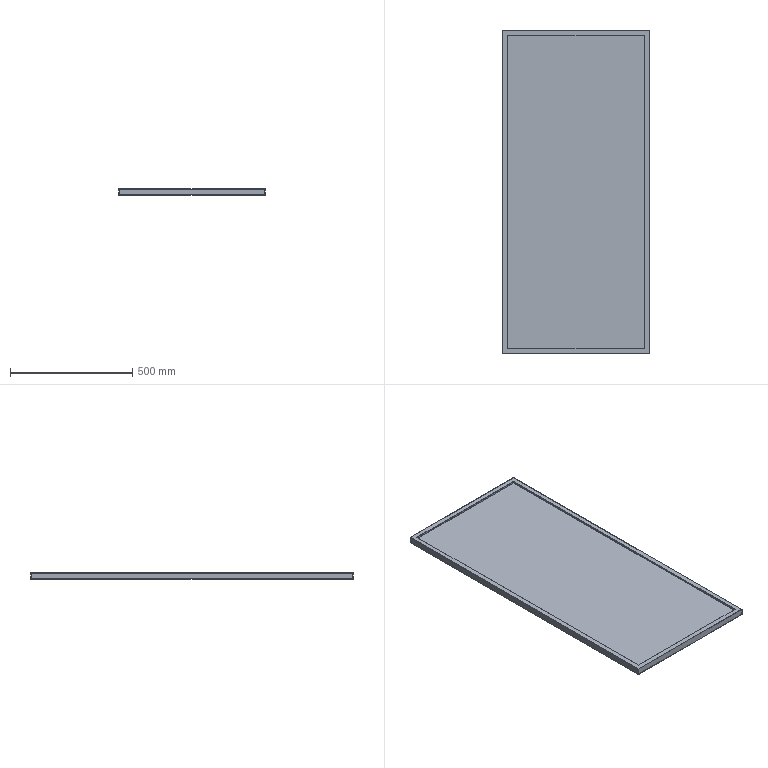Part | SolidWorks | features Extrusion 1, ICE 1, Shell 1 | 1 solid | 16 faces | box 598.5 x 1319 x 28 mm | volume 1912739 mm3 | plane 16
STEP:
#1=CARTESIAN_POINT('',(0.,1319.,28.));
#2=VERTEX_POINT('',#1);
#3=CARTESIAN_POINT('',(0.,0.,28.));
#4=VERTEX_POINT('',#3);
#5=CARTESIAN_POINT('',(0.,0.,28.));
#6=DIRECTION('',(0.,-1.,0.));
#7=VECTOR('',#6,1000.);
#8=LINE('',#5,#7);
#9=EDGE_CURVE('',#2,#4,#8,.T.);
#10=ORIENTED_EDGE('',*,*,#9,.T.);
#11=CARTESIAN_POINT('',(598.5,0.,28.));
#12=VERTEX_POINT('',#11);
#13=CARTESIAN_POINT('',(0.,0.,28.));
#14=DIRECTION('',(1.,0.,0.));
#15=VECTOR('',#14,1000.);
#16=LINE('',#13,#15);
#17=EDGE_CURVE('',#4,#12,#16,.T.);
#18=ORIENTED_EDGE('',*,*,#17,.T.);
#19=CARTESIAN_POINT('',(598.5,1319.,28.));
#20=VERTEX_POINT('',#19);
#21=CARTESIAN_POINT('',(598.5,0.,28.));
#22=DIRECTION('',(0.,1.,0.));
#23=VECTOR('',#22,1000.);
#24=LINE('',#21,#23);
#25=EDGE_CURVE('',#12,#20,#24,.T.);
#26=ORIENTED_EDGE('',*,*,#25,.T.);
#27=CARTESIAN_POINT('',(0.,1319.,28.));
#28=DIRECTION('',(-1.,0.,0.));
#29=VECTOR('',#28,1000.);
#30=LINE('',#27,#29);
#31=EDGE_CURVE('',#20,#2,#30,.T.);
#32=ORIENTED_EDGE('',*,*,#31,.T.);
#33=EDGE_LOOP('',(#10,#18,#26,#32));
#34=FACE_OUTER_BOUND('',#33,.T.);
#35=CARTESIAN_POINT('',(578.5,1299.,28.));
#36=VERTEX_POINT('',#35);
#37=CARTESIAN_POINT('',(20.,1299.,28.));
#38=VERTEX_POINT('',#37);
#39=CARTESIAN_POINT('',(578.5,1299.,28.));
#40=DIRECTION('',(-1.,0.,0.));
#41=VECTOR('',#40,1000.);
#42=LINE('',#39,#41);
#43=EDGE_CURVE('',#36,#38,#42,.T.);
#44=ORIENTED_EDGE('',*,*,#43,.F.);
#45=CARTESIAN_POINT('',(578.5,20.,28.));
#46=VERTEX_POINT('',#45);
#47=CARTESIAN_POINT('',(578.5,20.,28.));
#48=DIRECTION('',(0.,1.,0.));
#49=VECTOR('',#48,1000.);
#50=LINE('',#47,#49);
#51=EDGE_CURVE('',#46,#36,#50,.T.);
#52=ORIENTED_EDGE('',*,*,#51,.F.);
#53=CARTESIAN_POINT('',(20.,20.,28.));
#54=VERTEX_POINT('',#53);
#55=CARTESIAN_POINT('',(20.,20.,28.));
#56=DIRECTION('',(1.,0.,0.));
#57=VECTOR('',#56,1000.);
#58=LINE('',#55,#57);
#59=EDGE_CURVE('',#54,#46,#58,.T.);
#60=ORIENTED_EDGE('',*,*,#59,.F.);
#61=CARTESIAN_POINT('',(20.,1299.,28.));
#62=DIRECTION('',(0.,-1.,0.));
#63=VECTOR('',#62,1000.);
#64=LINE('',#61,#63);
#65=EDGE_CURVE('',#38,#54,#64,.T.);
#66=ORIENTED_EDGE('',*,*,#65,.F.);
#67=EDGE_LOOP('',(#44,#52,#60,#66));
#68=FACE_BOUND('',#67,.T.);
#69=CARTESIAN_POINT('',(0.,1319.,28.));
#70=DIRECTION('',(0.,0.,-1.));
#71=DIRECTION('',(-1.,0.,0.));
#72=AXIS2_PLACEMENT_3D('',#69,#70,#71);
#73=PLANE('',#72);
#74=ADVANCED_FACE('',(#34,#68),#73,.F.);
#75=CARTESIAN_POINT('',(0.,1319.,0.));
#76=VERTEX_POINT('',#75);
#77=CARTESIAN_POINT('',(0.,1319.,28.));
#78=DIRECTION('',(0.,0.,-1.));
#79=VECTOR('',#78,1000.);
#80=LINE('',#77,#79);
#81=EDGE_CURVE('',#2,#76,#80,.T.);
#82=ORIENTED_EDGE('',*,*,#81,.T.);
#83=CARTESIAN_POINT('',(0.,0.,0.));
#84=VERTEX_POINT('',#83);
#85=CARTESIAN_POINT('',(0.,0.,0.));
#86=DIRECTION('',(0.,-1.,0.));
#87=VECTOR('',#86,1000.);
#88=LINE('',#85,#87);
#89=EDGE_CURVE('',#76,#84,#88,.T.);
#90=ORIENTED_EDGE('',*,*,#89,.T.);
#91=CARTESIAN_POINT('',(0.,0.,28.));
#92=DIRECTION('',(0.,0.,-1.));
#93=VECTOR('',#92,1000.);
#94=LINE('',#91,#93);
#95=EDGE_CURVE('',#4,#84,#94,.T.);
#96=ORIENTED_EDGE('',*,*,#95,.F.);
#97=ORIENTED_EDGE('',*,*,#9,.F.);
#98=EDGE_LOOP('',(#82,#90,#96,#97));
#99=FACE_OUTER_BOUND('',#98,.T.);
#100=CARTESIAN_POINT('',(0.,0.,28.));
#101=DIRECTION('',(1.,0.,0.));
#102=DIRECTION('',(0.,0.,-1.));
#103=AXIS2_PLACEMENT_3D('',#100,#101,#102);
#104=PLANE('',#103);
#105=ADVANCED_FACE('',(#99),#104,.F.);
#106=ORIENTED_EDGE('',*,*,#95,.T.);
#107=CARTESIAN_POINT('',(598.5,0.,0.));
#108=VERTEX_POINT('',#107);
#109=CARTESIAN_POINT('',(0.,0.,0.));
#110=DIRECTION('',(1.,0.,0.));
#111=VECTOR('',#110,1000.);
#112=LINE('',#109,#111);
#113=EDGE_CURVE('',#84,#108,#112,.T.);
#114=ORIENTED_EDGE('',*,*,#113,.T.);
#115=CARTESIAN_POINT('',(598.5,0.,28.));
#116=DIRECTION('',(0.,0.,-1.));
#117=VECTOR('',#116,1000.);
#118=LINE('',#115,#117);
#119=EDGE_CURVE('',#12,#108,#118,.T.);
#120=ORIENTED_EDGE('',*,*,#119,.F.);
#121=ORIENTED_EDGE('',*,*,#17,.F.);
#122=EDGE_LOOP('',(#106,#114,#120,#121));
#123=FACE_OUTER_BOUND('',#122,.T.);
#124=CARTESIAN_POINT('',(0.,0.,28.));
#125=DIRECTION('',(0.,1.,0.));
#126=DIRECTION('',(0.,0.,1.));
#127=AXIS2_PLACEMENT_3D('',#124,#125,#126);
#128=PLANE('',#127);
#129=ADVANCED_FACE('',(#123),#128,.F.);
#130=ORIENTED_EDGE('',*,*,#119,.T.);
#131=CARTESIAN_POINT('',(598.5,1319.,0.));
#132=VERTEX_POINT('',#131);
#133=CARTESIAN_POINT('',(598.5,0.,0.));
#134=DIRECTION('',(0.,1.,0.));
#135=VECTOR('',#134,1000.);
#136=LINE('',#133,#135);
#137=EDGE_CURVE('',#108,#132,#136,.T.);
#138=ORIENTED_EDGE('',*,*,#137,.T.);
#139=CARTESIAN_POINT('',(598.5,1319.,28.));
#140=DIRECTION('',(0.,0.,-1.));
#141=VECTOR('',#140,1000.);
#142=LINE('',#139,#141);
#143=EDGE_CURVE('',#20,#132,#142,.T.);
#144=ORIENTED_EDGE('',*,*,#143,.F.);
#145=ORIENTED_EDGE('',*,*,#25,.F.);
#146=EDGE_LOOP('',(#130,#138,#144,#145));
#147=FACE_OUTER_BOUND('',#146,.T.);
#148=CARTESIAN_POINT('',(598.5,0.,28.));
#149=DIRECTION('',(-1.,0.,0.));
#150=DIRECTION('',(0.,0.,1.));
#151=AXIS2_PLACEMENT_3D('',#148,#149,#150);
#152=PLANE('',#151);
#153=ADVANCED_FACE('',(#147),#152,.F.);
#154=ORIENTED_EDGE('',*,*,#143,.T.);
#155=CARTESIAN_POINT('',(0.,1319.,0.));
#156=DIRECTION('',(-1.,0.,0.));
#157=VECTOR('',#156,1000.);
#158=LINE('',#155,#157);
#159=EDGE_CURVE('',#132,#76,#158,.T.);
#160=ORIENTED_EDGE('',*,*,#159,.T.);
#161=ORIENTED_EDGE('',*,*,#81,.F.);
#162=ORIENTED_EDGE('',*,*,#31,.F.);
#163=EDGE_LOOP('',(#154,#160,#161,#162));
#164=FACE_OUTER_BOUND('',#163,.T.);
#165=CARTESIAN_POINT('',(0.,1319.,28.));
#166=DIRECTION('',(0.,-1.,0.));
#167=DIRECTION('',(0.,0.,-1.));
#168=AXIS2_PLACEMENT_3D('',#165,#166,#167);
#169=PLANE('',#168);
#170=ADVANCED_FACE('',(#164),#169,.F.);
#171=ORIENTED_EDGE('',*,*,#89,.F.);
#172=ORIENTED_EDGE('',*,*,#159,.F.);
#173=ORIENTED_EDGE('',*,*,#137,.F.);
#174=ORIENTED_EDGE('',*,*,#113,.F.);
#175=EDGE_LOOP('',(#171,#172,#173,#174));
#176=FACE_OUTER_BOUND('',#175,.T.);
#177=CARTESIAN_POINT('',(0.,1319.,0.));
#178=DIRECTION('',(0.,0.,-1.));
#179=DIRECTION('',(-1.,0.,0.));
#180=AXIS2_PLACEMENT_3D('',#177,#178,#179);
#181=PLANE('',#180);
#182=ADVANCED_FACE('',(#176),#181,.T.);
#183=CARTESIAN_POINT('',(2.,1317.,26.));
#184=VERTEX_POINT('',#183);
#185=CARTESIAN_POINT('',(2.,2.,26.));
#186=VERTEX_POINT('',#185);
#187=CARTESIAN_POINT('',(2.,0.,26.));
#188=DIRECTION('',(0.,-1.,0.));
#189=VECTOR('',#188,1000.);
#190=LINE('',#187,#189);
#191=EDGE_CURVE('',#184,#186,#190,.T.);
#192=ORIENTED_EDGE('',*,*,#191,.F.);
#193=CARTESIAN_POINT('',(596.5,1317.,26.));
#194=VERTEX_POINT('',#193);
#195=CARTESIAN_POINT('',(0.,1317.,26.));
#196=DIRECTION('',(-1.,0.,0.));
#197=VECTOR('',#196,1000.);
#198=LINE('',#195,#197);
#199=EDGE_CURVE('',#194,#184,#198,.T.);
#200=ORIENTED_EDGE('',*,*,#199,.F.);
#201=CARTESIAN_POINT('',(596.5,2.,26.));
#202=VERTEX_POINT('',#201);
#203=CARTESIAN_POINT('',(596.5,0.,26.));
#204=DIRECTION('',(0.,1.,0.));
#205=VECTOR('',#204,1000.);
#206=LINE('',#203,#205);
#207=EDGE_CURVE('',#202,#194,#206,.T.);
#208=ORIENTED_EDGE('',*,*,#207,.F.);
#209=CARTESIAN_POINT('',(0.,2.,26.));
#210=DIRECTION('',(1.,0.,0.));
#211=VECTOR('',#210,1000.);
#212=LINE('',#209,#211);
#213=EDGE_CURVE('',#186,#202,#212,.T.);
#214=ORIENTED_EDGE('',*,*,#213,.F.);
#215=EDGE_LOOP('',(#192,#200,#208,#214));
#216=FACE_OUTER_BOUND('',#215,.T.);
#217=CARTESIAN_POINT('',(578.5,20.,26.));
#218=VERTEX_POINT('',#217);
#219=CARTESIAN_POINT('',(578.5,1299.,26.));
#220=VERTEX_POINT('',#219);
#221=CARTESIAN_POINT('',(578.5,20.,26.));
#222=DIRECTION('',(0.,1.,0.));
#223=VECTOR('',#222,1000.);
#224=LINE('',#221,#223);
#225=EDGE_CURVE('',#218,#220,#224,.T.);
#226=ORIENTED_EDGE('',*,*,#225,.T.);
#227=CARTESIAN_POINT('',(20.,1299.,26.));
#228=VERTEX_POINT('',#227);
#229=CARTESIAN_POINT('',(578.5,1299.,26.));
#230=DIRECTION('',(-1.,0.,0.));
#231=VECTOR('',#230,1000.);
#232=LINE('',#229,#231);
#233=EDGE_CURVE('',#220,#228,#232,.T.);
#234=ORIENTED_EDGE('',*,*,#233,.T.);
#235=CARTESIAN_POINT('',(20.,20.,26.));
#236=VERTEX_POINT('',#235);
#237=CARTESIAN_POINT('',(20.,1299.,26.));
#238=DIRECTION('',(0.,-1.,0.));
#239=VECTOR('',#238,1000.);
#240=LINE('',#237,#239);
#241=EDGE_CURVE('',#228,#236,#240,.T.);
#242=ORIENTED_EDGE('',*,*,#241,.T.);
#243=CARTESIAN_POINT('',(20.,20.,26.));
#244=DIRECTION('',(1.,0.,0.));
#245=VECTOR('',#244,1000.);
#246=LINE('',#243,#245);
#247=EDGE_CURVE('',#236,#218,#246,.T.);
#248=ORIENTED_EDGE('',*,*,#247,.T.);
#249=EDGE_LOOP('',(#226,#234,#242,#248));
#250=FACE_BOUND('',#249,.T.);
#251=CARTESIAN_POINT('',(0.,1319.,26.));
#252=DIRECTION('',(0.,0.,1.));
#253=DIRECTION('',(1.,0.,0.));
#254=AXIS2_PLACEMENT_3D('',#251,#252,#253);
#255=PLANE('',#254);
#256=ADVANCED_FACE('',(#216,#250),#255,.F.);
#257=ORIENTED_EDGE('',*,*,#43,.T.);
#258=CARTESIAN_POINT('',(20.,1299.,26.));
#259=DIRECTION('',(0.,0.,1.));
#260=VECTOR('',#259,1000.);
#261=LINE('',#258,#260);
#262=EDGE_CURVE('',#228,#38,#261,.T.);
#263=ORIENTED_EDGE('',*,*,#262,.F.);
#264=ORIENTED_EDGE('',*,*,#233,.F.);
#265=CARTESIAN_POINT('',(578.5,1299.,26.));
#266=DIRECTION('',(0.,0.,1.));
#267=VECTOR('',#266,1000.);
#268=LINE('',#265,#267);
#269=EDGE_CURVE('',#220,#36,#268,.T.);
#270=ORIENTED_EDGE('',*,*,#269,.T.);
#271=EDGE_LOOP('',(#257,#263,#264,#270));
#272=FACE_OUTER_BOUND('',#271,.T.);
#273=CARTESIAN_POINT('',(578.5,1299.,26.));
#274=DIRECTION('',(0.,1.,0.));
#275=DIRECTION('',(0.,0.,1.));
#276=AXIS2_PLACEMENT_3D('',#273,#274,#275);
#277=PLANE('',#276);
#278=ADVANCED_FACE('',(#272),#277,.F.);
#279=ORIENTED_EDGE('',*,*,#51,.T.);
#280=ORIENTED_EDGE('',*,*,#269,.F.);
#281=ORIENTED_EDGE('',*,*,#225,.F.);
#282=CARTESIAN_POINT('',(578.5,20.,26.));
#283=DIRECTION('',(0.,0.,1.));
#284=VECTOR('',#283,1000.);
#285=LINE('',#282,#284);
#286=EDGE_CURVE('',#218,#46,#285,.T.);
#287=ORIENTED_EDGE('',*,*,#286,.T.);
#288=EDGE_LOOP('',(#279,#280,#281,#287));
#289=FACE_OUTER_BOUND('',#288,.T.);
#290=CARTESIAN_POINT('',(578.5,20.,26.));
#291=DIRECTION('',(1.,0.,0.));
#292=DIRECTION('',(0.,0.,-1.));
#293=AXIS2_PLACEMENT_3D('',#290,#291,#292);
#294=PLANE('',#293);
#295=ADVANCED_FACE('',(#289),#294,.F.);
#296=ORIENTED_EDGE('',*,*,#59,.T.);
#297=ORIENTED_EDGE('',*,*,#286,.F.);
#298=ORIENTED_EDGE('',*,*,#247,.F.);
#299=CARTESIAN_POINT('',(20.,20.,26.));
#300=DIRECTION('',(0.,0.,1.));
#301=VECTOR('',#300,1000.);
#302=LINE('',#299,#301);
#303=EDGE_CURVE('',#236,#54,#302,.T.);
#304=ORIENTED_EDGE('',*,*,#303,.T.);
#305=EDGE_LOOP('',(#296,#297,#298,#304));
#306=FACE_OUTER_BOUND('',#305,.T.);
#307=CARTESIAN_POINT('',(20.,20.,26.));
#308=DIRECTION('',(0.,-1.,0.));
#309=DIRECTION('',(0.,0.,-1.));
#310=AXIS2_PLACEMENT_3D('',#307,#308,#309);
#311=PLANE('',#310);
#312=ADVANCED_FACE('',(#306),#311,.F.);
#313=ORIENTED_EDGE('',*,*,#65,.T.);
#314=ORIENTED_EDGE('',*,*,#303,.F.);
#315=ORIENTED_EDGE('',*,*,#241,.F.);
#316=ORIENTED_EDGE('',*,*,#262,.T.);
#317=EDGE_LOOP('',(#313,#314,#315,#316));
#318=FACE_OUTER_BOUND('',#317,.T.);
#319=CARTESIAN_POINT('',(20.,1299.,26.));
#320=DIRECTION('',(-1.,0.,0.));
#321=DIRECTION('',(0.,0.,1.));
#322=AXIS2_PLACEMENT_3D('',#319,#320,#321);
#323=PLANE('',#322);
#324=ADVANCED_FACE('',(#318),#323,.F.);
#325=CARTESIAN_POINT('',(2.,1317.,2.));
#326=VERTEX_POINT('',#325);
#327=CARTESIAN_POINT('',(2.,2.,2.));
#328=VERTEX_POINT('',#327);
#329=CARTESIAN_POINT('',(2.,1319.,2.));
#330=DIRECTION('',(0.,-1.,0.));
#331=VECTOR('',#330,1000.);
#332=LINE('',#329,#331);
#333=EDGE_CURVE('',#326,#328,#332,.T.);
#334=ORIENTED_EDGE('',*,*,#333,.T.);
#335=CARTESIAN_POINT('',(596.5,2.,2.));
#336=VERTEX_POINT('',#335);
#337=CARTESIAN_POINT('',(0.,2.,2.));
#338=DIRECTION('',(1.,0.,0.));
#339=VECTOR('',#338,1000.);
#340=LINE('',#337,#339);
#341=EDGE_CURVE('',#328,#336,#340,.T.);
#342=ORIENTED_EDGE('',*,*,#341,.T.);
#343=CARTESIAN_POINT('',(596.5,1317.,2.));
#344=VERTEX_POINT('',#343);
#345=CARTESIAN_POINT('',(596.5,1319.,2.));
#346=DIRECTION('',(0.,1.,0.));
#347=VECTOR('',#346,1000.);
#348=LINE('',#345,#347);
#349=EDGE_CURVE('',#336,#344,#348,.T.);
#350=ORIENTED_EDGE('',*,*,#349,.T.);
#351=CARTESIAN_POINT('',(0.,1317.,2.));
#352=DIRECTION('',(-1.,0.,0.));
#353=VECTOR('',#352,1000.);
#354=LINE('',#351,#353);
#355=EDGE_CURVE('',#344,#326,#354,.T.);
#356=ORIENTED_EDGE('',*,*,#355,.T.);
#357=EDGE_LOOP('',(#334,#342,#350,#356));
#358=FACE_OUTER_BOUND('',#357,.T.);
#359=CARTESIAN_POINT('',(0.,1319.,2.));
#360=DIRECTION('',(0.,0.,-1.));
#361=DIRECTION('',(-1.,0.,0.));
#362=AXIS2_PLACEMENT_3D('',#359,#360,#361);
#363=PLANE('',#362);
#364=ADVANCED_FACE('',(#358),#363,.F.);
#365=CARTESIAN_POINT('',(596.5,1317.,28.));
#366=DIRECTION('',(0.,0.,-1.));
#367=VECTOR('',#366,1000.);
#368=LINE('',#365,#367);
#369=EDGE_CURVE('',#194,#344,#368,.T.);
#370=ORIENTED_EDGE('',*,*,#369,.F.);
#371=ORIENTED_EDGE('',*,*,#199,.T.);
#372=CARTESIAN_POINT('',(2.,1317.,28.));
#373=DIRECTION('',(0.,0.,-1.));
#374=VECTOR('',#373,1000.);
#375=LINE('',#372,#374);
#376=EDGE_CURVE('',#184,#326,#375,.T.);
#377=ORIENTED_EDGE('',*,*,#376,.T.);
#378=ORIENTED_EDGE('',*,*,#355,.F.);
#379=EDGE_LOOP('',(#370,#371,#377,#378));
#380=FACE_OUTER_BOUND('',#379,.T.);
#381=CARTESIAN_POINT('',(0.,1317.,28.));
#382=DIRECTION('',(0.,-1.,0.));
#383=DIRECTION('',(0.,0.,-1.));
#384=AXIS2_PLACEMENT_3D('',#381,#382,#383);
#385=PLANE('',#384);
#386=ADVANCED_FACE('',(#380),#385,.T.);
#387=CARTESIAN_POINT('',(596.5,2.,28.));
#388=DIRECTION('',(0.,0.,-1.));
#389=VECTOR('',#388,1000.);
#390=LINE('',#387,#389);
#391=EDGE_CURVE('',#202,#336,#390,.T.);
#392=ORIENTED_EDGE('',*,*,#391,.F.);
#393=ORIENTED_EDGE('',*,*,#207,.T.);
#394=ORIENTED_EDGE('',*,*,#369,.T.);
#395=ORIENTED_EDGE('',*,*,#349,.F.);
#396=EDGE_LOOP('',(#392,#393,#394,#395));
#397=FACE_OUTER_BOUND('',#396,.T.);
#398=CARTESIAN_POINT('',(596.5,0.,28.));
#399=DIRECTION('',(-1.,0.,0.));
#400=DIRECTION('',(0.,0.,1.));
#401=AXIS2_PLACEMENT_3D('',#398,#399,#400);
#402=PLANE('',#401);
#403=ADVANCED_FACE('',(#397),#402,.T.);
#404=CARTESIAN_POINT('',(2.,2.,28.));
#405=DIRECTION('',(0.,0.,-1.));
#406=VECTOR('',#405,1000.);
#407=LINE('',#404,#406);
#408=EDGE_CURVE('',#186,#328,#407,.T.);
#409=ORIENTED_EDGE('',*,*,#408,.F.);
#410=ORIENTED_EDGE('',*,*,#213,.T.);
#411=ORIENTED_EDGE('',*,*,#391,.T.);
#412=ORIENTED_EDGE('',*,*,#341,.F.);
#413=EDGE_LOOP('',(#409,#410,#411,#412));
#414=FACE_OUTER_BOUND('',#413,.T.);
#415=CARTESIAN_POINT('',(0.,2.,28.));
#416=DIRECTION('',(0.,1.,0.));
#417=DIRECTION('',(0.,0.,1.));
#418=AXIS2_PLACEMENT_3D('',#415,#416,#417);
#419=PLANE('',#418);
#420=ADVANCED_FACE('',(#414),#419,.T.);
#421=ORIENTED_EDGE('',*,*,#376,.F.);
#422=ORIENTED_EDGE('',*,*,#191,.T.);
#423=ORIENTED_EDGE('',*,*,#408,.T.);
#424=ORIENTED_EDGE('',*,*,#333,.F.);
#425=EDGE_LOOP('',(#421,#422,#423,#424));
#426=FACE_OUTER_BOUND('',#425,.T.);
#427=CARTESIAN_POINT('',(2.,0.,28.));
#428=DIRECTION('',(1.,0.,0.));
#429=DIRECTION('',(0.,0.,-1.));
#430=AXIS2_PLACEMENT_3D('',#427,#428,#429);
#431=PLANE('',#430);
#432=ADVANCED_FACE('',(#426),#431,.T.);
#433=CLOSED_SHELL('',(#74,#105,#129,#153,#170,#182,#256,#278,#295,#312,#324,#364,#386,#403,#420,#432));
#434=MANIFOLD_SOLID_BREP('',#433);
#435=CARTESIAN_POINT('',(0.,0.,0.));
#436=DIRECTION('',(0.,0.,1.));
#437=DIRECTION('',(1.,0.,0.));
#438=AXIS2_PLACEMENT_3D('',#435,#436,#437);
#439=(LENGTH_UNIT()NAMED_UNIT(*)SI_UNIT(.MILLI.,.METRE.));
#440=UNCERTAINTY_MEASURE_WITH_UNIT(LENGTH_MEASURE(0.00001),#439,'','');
#441=(NAMED_UNIT(*)PLANE_ANGLE_UNIT()SI_UNIT($,.RADIAN.));
#442=(NAMED_UNIT(*)SI_UNIT($,.STERADIAN.)SOLID_ANGLE_UNIT());
#443=(GEOMETRIC_REPRESENTATION_CONTEXT(3)GLOBAL_UNCERTAINTY_ASSIGNED_CONTEXT((#440))GLOBAL_UNIT_ASSIGNED_CONTEXT((#439,#441,#442))REPRESENTATION_CONTEXT('',''));
#444=ADVANCED_BREP_SHAPE_REPRESENTATION('',(#434,#438),#443);